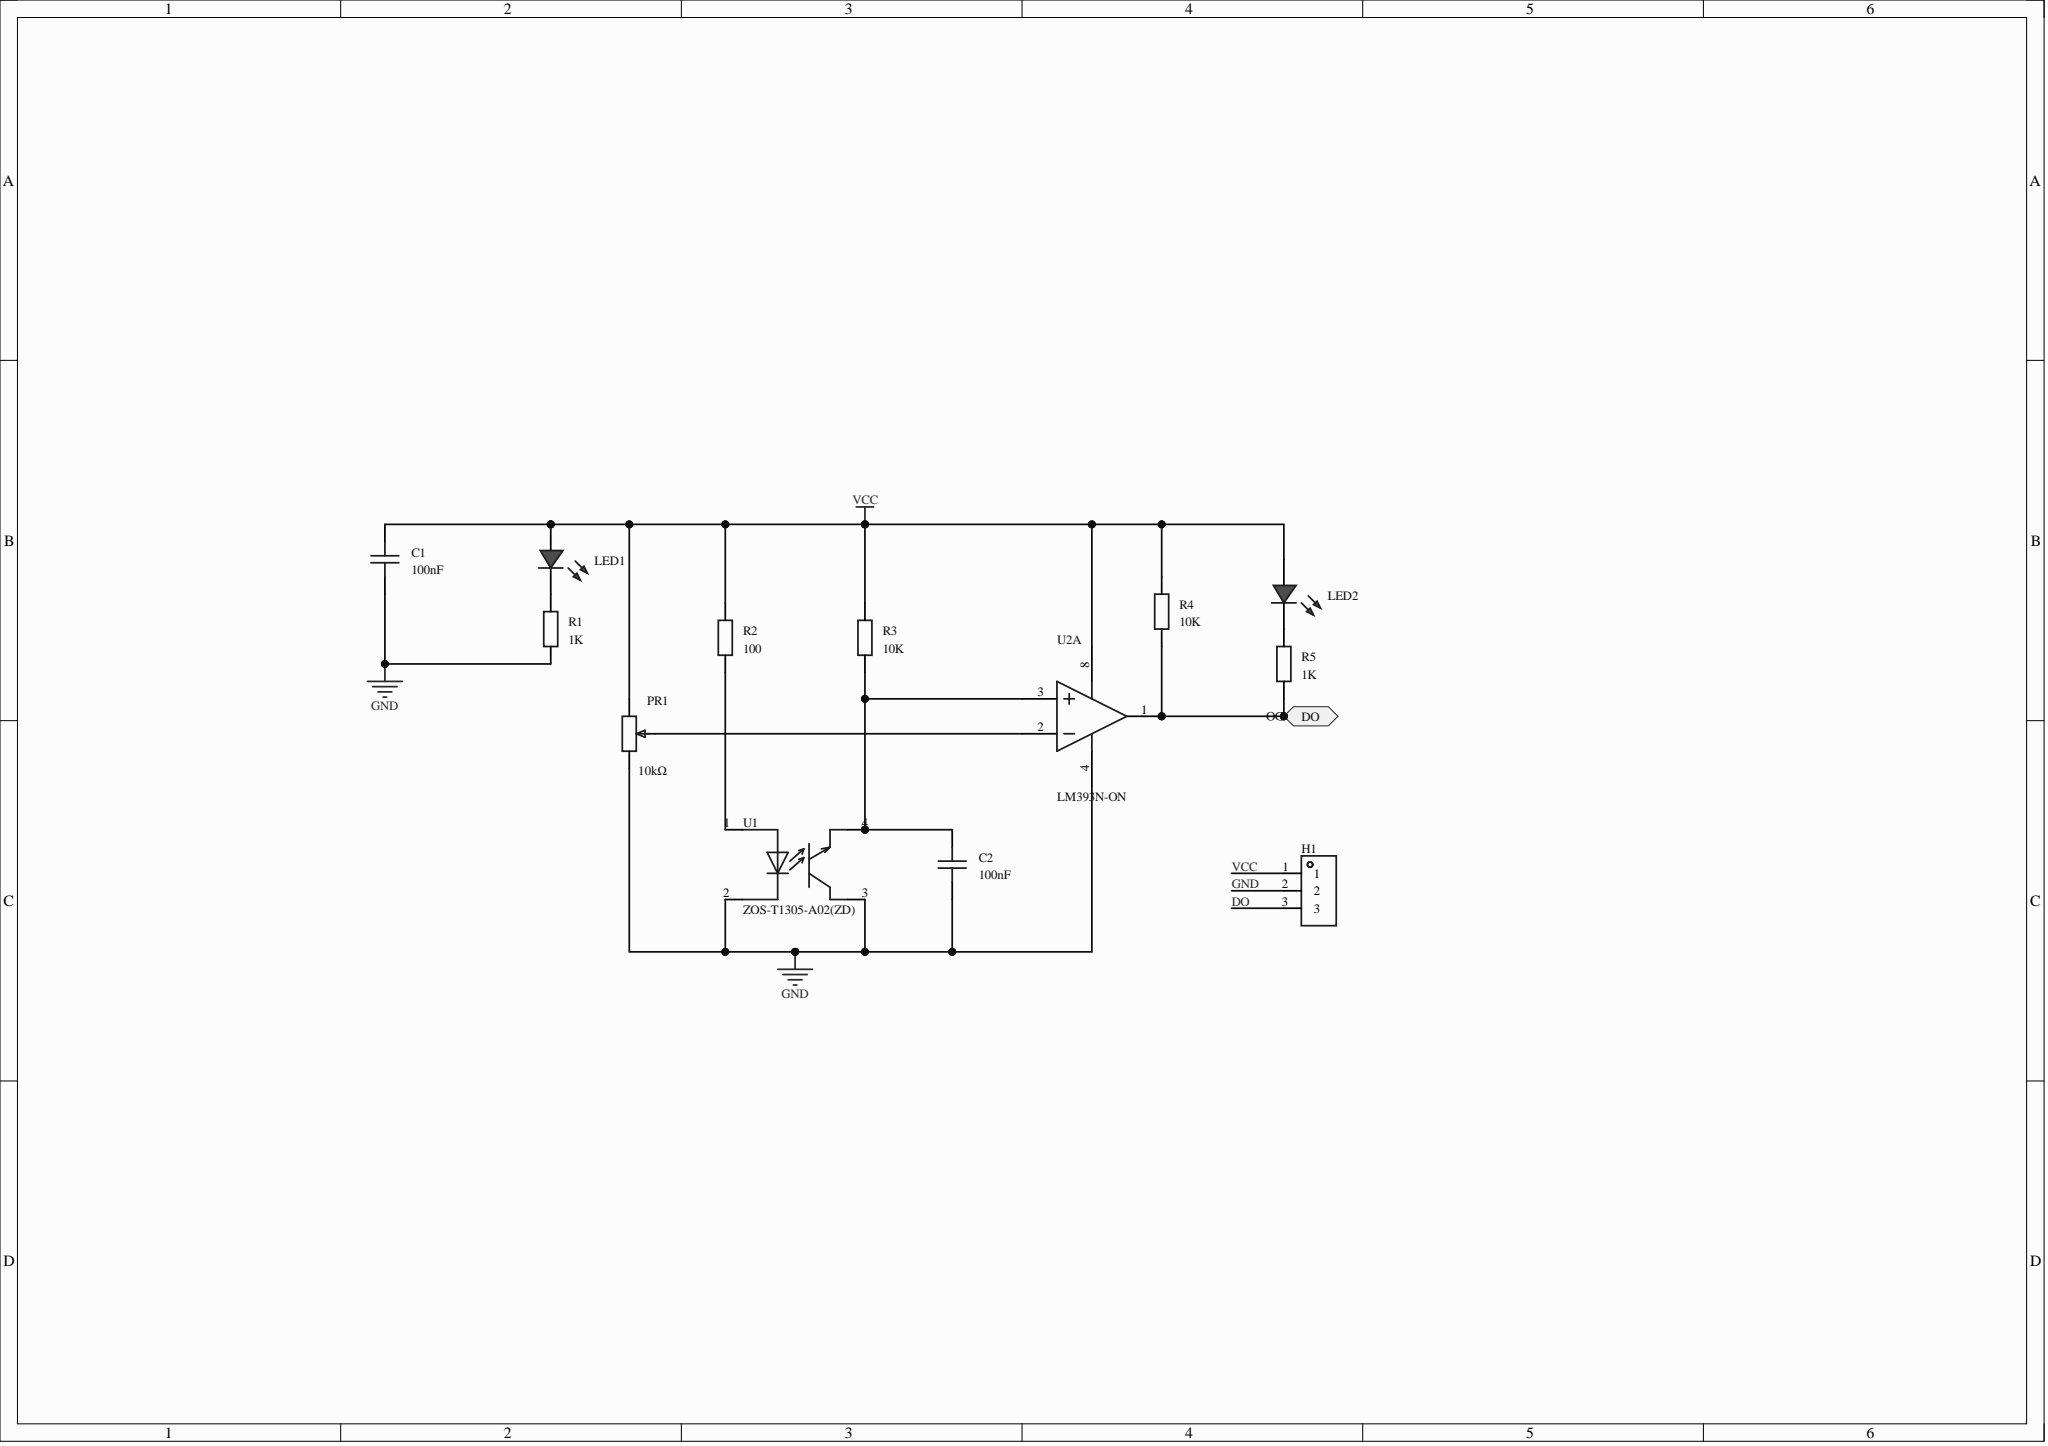Circuit board | Altium Designer | 13 parts | 8 nets
Bill of materials:
Comment,Description,Designator,Footprint,LibRef,Quantity
"100nF","","C1, C2","C0603","CAP_0603","2"
"","","H1","HDR-TH_3P-P2.54-V-M","HDR-M_2.54_1x3P","1"
"","","LED1, LED2","LED_TH-3mm","LED_TH-R_3mm","2"
"10kΩ","","PR1","R_3296","R_3296","1"
"1K","","R1, R5","R0603","Res_0603","2"
"100","","R2","R0603","Res_0603","1"
"10K","","R3, R4","R0603","Res_0603","2"
"ZOS-T1305-A02(ZD)","槽宽:5.2mm;暗电流:100nA;峰值波长:940nm;正向压降(Vf):1.2V;","U1","OPTO-TH_ZOS-T1305-A02","ZOS-T1305-A02(ZD)","1"
"LM393N-ON","输入失调电压(Vos):5mV;输入偏置电流(Ib):250nA;","U2","PDIP-8_L9.6-W6.4-P2.54-LS7.9-BL","LM393N-ON","1"
Netlist (Protel format):
[
C1
C0603
100nF



]
[
C2
C0603
100nF



]
[
H1
HDR-TH_3P-P2.54-V-M




]
[
LED1
LED_TH-3mm




]
[
LED2
LED_TH-3mm




]
[
PR1
R_3296
10kΩ



]
[
R1
R0603
1K



]
[
R2
R0603
100



]
[
R3
R0603
10K



]
[
R4
R0603
10K



]
[
R5
R0603
1K



]
[
U1
OPTO-TH_ZOS-T1305-A02
ZOS-T1305-A02(ZD)



]
[
U2
PDIP-8_L9.6-W6.4-P2.54-LS7.9-BL
LM393N-ON



]
(
VCC
C1-2
H1-1
LED1-1
LED2-1
PR1-3
R2-2
R3-2
R4-2
U2-8
)
(
NetR2_1
R2-1
U1-1
)
(
NetPR1_2
PR1-2
U2-2
)
(
NetLED2_2
LED2-2
R5-2
)
(
NetLED1_2
LED1-2
R1-2
)
(
NetC2_2
C2-2
R3-1
U1-4
U2-3
)
(
GND
C1-1
C2-1
H1-2
PR1-1
R1-1
U1-2
U1-3
U2-4
)
(
DO
H1-3
R4-1
R5-1
U2-1
)